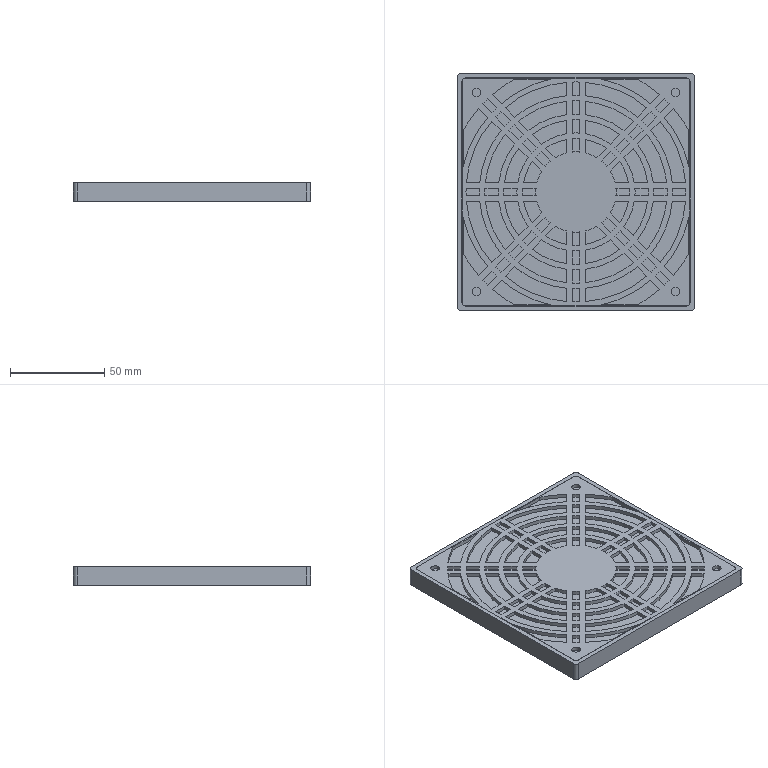Part | SolidWorks | features ICE 6, BossThin 3, Fillet 3, CirPattern 1, CutThin 1, Extrusion 1, RefAxis 1 | 3 solids | 671 faces | box 125.5 x 125.5 x 10 mm | volume 129712 mm3 | cylinder 344 | plane 327 | commonest cylinder face diameters 42.5 x34 56.5 x34 62.5 x34 76.5 x34 82.5 x34 96.5 x34